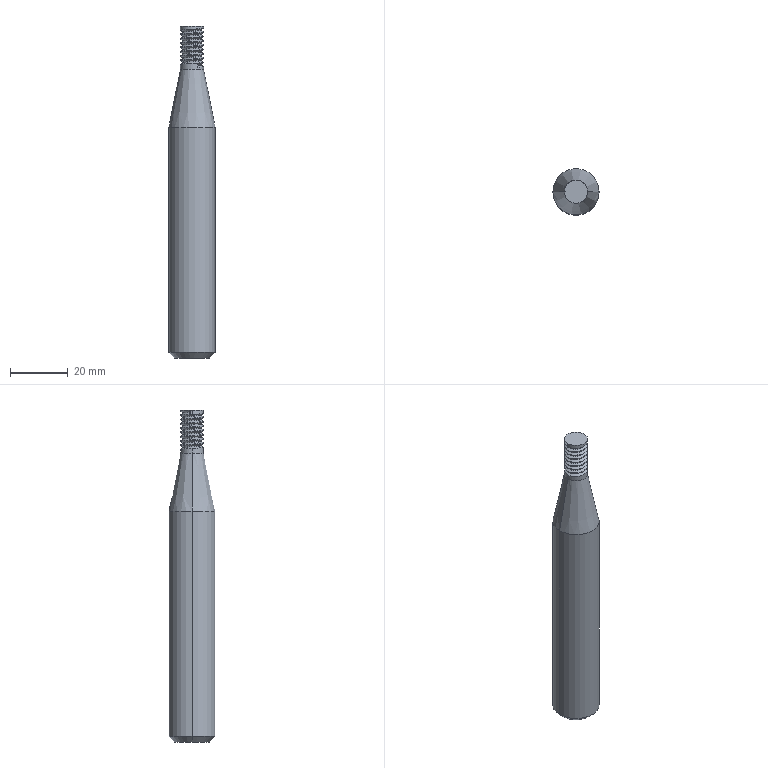Part | SolidWorks | features Chamfer 2, Extrusion 1, ICE 1, SweepThread 1 | 1 solid | 32 faces | box 16 x 16 x 115 mm | volume 18955 mm3 | cylinder 21 | cone 4 | plane 4 | spline 3 | commonest cylinder face diameters 8 x19 16 x2